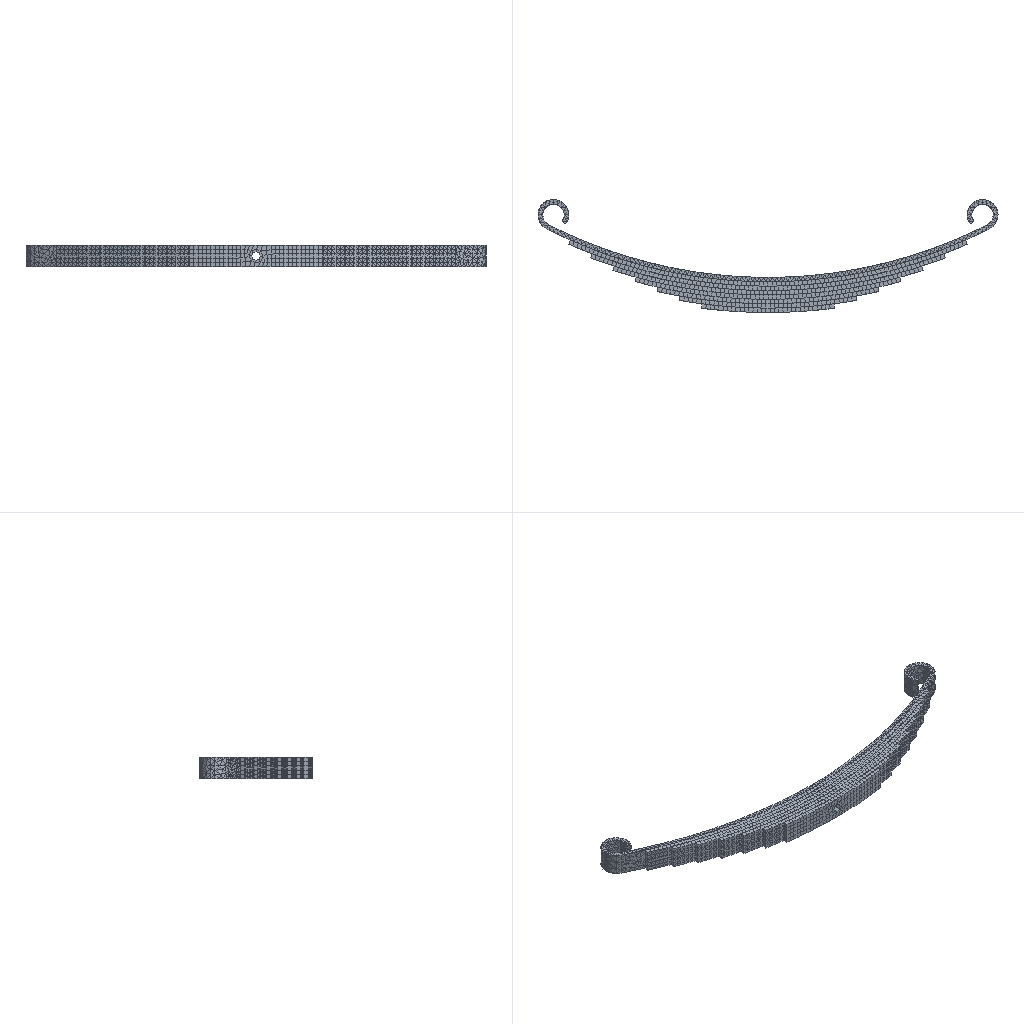Simulation study | ansys workbench
Set-up summary:
category,name,step,type,value,unit,region
solver,ansys_workbench
units,mm-N-s-tonne (MPa),,stated,"/units,MPA"
analysis,LS1,,static
load_step,LS1,LS1,static,nsubst=1; time=1
mesh,nodes,,,25414
mesh,elements,,,15995
element_type,TARGE170,,,5078
element_type,CONTA174,,,5078
element_type,SOLID187,,,3507
element_type,SOLID186,,,2176
element_type,SURF154,,,156
material,Structural Steel,,E,200000,tonne s^-2 mm^-1
material,Structural Steel,,nu,0.3
material,Structural Steel,,density,7.85e-09,tonne mm^-3
material,Structural Steel,,conductivity,60.5,tonne mm s^-3 C^-1
material,Structural Steel,,specific_heat,4.34e+08,mm^2 s^-2 C^-1
material,Structural Steel,,cte,1.2e-05,C^-1
material,Structural Steel,,permeability,10000
material,Structural Steel,,resistivity,0.00017,ohm mm
load,Define Force Using Surface Effect Elements,LS1,surface-effect pres face 2,3.366,,SURF154 #23
bc,Fixed Supports,model,fixed,[dofs=ALL],,_FIXEDSU
bc,Frictionless Supports X,model,fixed,[dofs=UX],,_FRICSUX
bc,Frictionless Supports Y,model,fixed,[dofs=UY],,_FRICSUY
bc,Frictionless Supports Z,model,fixed,[dofs=UZ],,_FRICSUZ
contact,No Separation - 8 To 7,,no separation (always),element=CONTA174
contact,No Separation - 7 To 6,,no separation (always),element=CONTA174
contact,No Separation - 6 To 5,,no separation (always),element=CONTA174
contact,No Separation - 5 To 4,,no separation (always),element=CONTA174
contact,No Separation - 4 To 3,,no separation (always),element=CONTA174
contact,No Separation - 3 To 2,,no separation (always),element=CONTA174
contact,No Separation - 2 To 1,,no separation (always),element=CONTA174
named_set,_FIXEDSU,,node,466
named_set,_FRICSUX,,node,328
named_set,_FRICSUY,,node,96
named_set,_FRICSUZ,,node,232
Ansys APDL input file, long lists of numbers shortened:
/batch
/config,noeldb,1     ! force off writing results to database
*get,_wallstrt,active,,time,wall
! ANSYS input file written by Workbench version 19.0 RELEASE
! File used for geometry attach:
/title,unsaved_project--Static Structural (A5)
*DIM,_wb_ProjectScratch_dir,string,248
_wb_ProjectScratch_dir(1) = ''
*DIM,_wb_SolverFiles_dir,string,248
_wb_SolverFiles_dir(1) = ''
*DIM,_wb_userfiles_dir,string,248
_wb_userfiles_dir(1) = ''
/com,--- Data in consistent NMM units. See Solving Units in the help system for more information.
/units,MPA
/nopr
/wb,file,start              !  signify a WB generated input file
/prep7
! Turn off shape checking because checks already performed inside WB mesher.
! See help system for more information.
SHPP,OFF,,NOWARN
/nolist
etcon,set             ! allow ANSYS to choose best KEYOP's for 180x elements
/com,*********** Nodes for the whole assembly ***********
nblock,3,,27955
(1i9,3e20.9e3)
        1    2.672589323E+001   -5.969305683E+001   -5.813771560E+000
! (25413 more lines like these left out)
-1
/wb,elem,start            !  set before creation of elements
/com,*********** Elements for Body 1 "8" ***********
et,1,186
keyo,1,2,1          ! set full integration on SOLID186
eblock,19,solid,,156
(19i9)
        1        1        1        1        0        0        0        0       20        0      207     1697     1698     1718     1761     1920     1919     1899     1856
! (311 more lines like these left out)
-1
/com,*********** Elements for Body 2 "7" ***********
et,2,186
keyo,2,2,1          ! set full integration on SOLID186
eblock,19,solid,,206
(19i9)
        2        2        2        2        0        0        0        0       20        0        1        5        6       31       89      308      307      282      224
! (411 more lines like these left out)
-1
/com,*********** Elements for Body 3 "6" ***********
et,3,186
keyo,3,2,1          ! set full integration on SOLID186
eblock,19,solid,,256
(19i9)
        3        3        3        3        0        0        0        0       20        0     1033     8429     8430     8460     8533     8812     8811     8781     8708
! (511 more lines like these left out)
-1
/com,*********** Elements for Body 4 "5" ***********
et,4,186
keyo,4,2,1          ! set full integration on SOLID186
eblock,19,solid,,312
(19i9)
        4        4        4        4        0        0        0        0       20        0      363     2992     3028     3170     3748     3457     3421     3279     3465
! (623 more lines like these left out)
-1
/com,*********** Elements for Body 5 "4" ***********
et,5,186
keyo,5,2,1          ! set full integration on SOLID186
eblock,19,solid,,358
(19i9)
        5        5        5        5        0        0        0        0       20        0      675     5520     5794     5521     5665     6069     5795     6068     5924
! (715 more lines like these left out)
-1
/com,*********** Elements for Body 6 "3" ***********
et,6,186
keyo,6,2,1          ! set full integration on SOLID186
eblock,19,solid,,416
(19i9)
        6        6        6        6        0        0        0        0       20        0     4796    18236    18405    18365    18366    18877    18708    18748    18747
! (831 more lines like these left out)
-1
/com,*********** Elements for Body 7 "2" ***********
et,7,186
keyo,7,2,1          ! set full integration on SOLID186
eblock,19,solid,,472
(19i9)
        7        7        7        7        0        0        0        0       20        0     5212    21601    21605    21847    21750    22336    22332    22090    22187
! (943 more lines like these left out)
-1
/com,*********** Elements for Body 8 "1" ***********
et,8,187
eblock,19,solid,,3507
(19i9)
        8        8        8        8        0        0        0        0       10        0     1289    11163    11667    11316    11265    15185    16145    15182    15181
! (7013 more lines like these left out)
-1
/wb,elem,end               !  done creating elements
/com,*********** Send User Defined Coordinate System(s) ***********
csys,0
toffst,273.15,  ! Temperature offset from absolute zero
/com,*********** Set Reference Temperature ***********
tref,22.
/wb,mat,start              !  starting to send materials
/com,*********** Send Materials ***********
Temperature = 'TEMP' ! Temperature
MP,DENS,1,7.85e-09,	! tonne mm^-3
MP,ALPX,1,1.2e-05,	! C^-1
MP,C,1,434000000,	! mm^2 s^-2 C^-1
MP,KXX,1,60.5,	! tonne mm s^-3 C^-1
MP,RSVX,1,0.00017,	! ohm mm
MP,EX,1,200000,	! tonne s^-2 mm^-1
MP,NUXY,1,0.3,
MP,MURX,1,10000,
Temperature = 'TEMP' ! Temperature
MP,DENS,2,7.85e-09,	! tonne mm^-3
MP,ALPX,2,1.2e-05,	! C^-1
MP,C,2,434000000,	! mm^2 s^-2 C^-1
MP,KXX,2,60.5,	! tonne mm s^-3 C^-1
MP,RSVX,2,0.00017,	! ohm mm
MP,EX,2,200000,	! tonne s^-2 mm^-1
MP,NUXY,2,0.3,
MP,MURX,2,10000,
Temperature = 'TEMP' ! Temperature
MP,DENS,3,7.85e-09,	! tonne mm^-3
MP,ALPX,3,1.2e-05,	! C^-1
MP,C,3,434000000,	! mm^2 s^-2 C^-1
MP,KXX,3,60.5,	! tonne mm s^-3 C^-1
MP,RSVX,3,0.00017,	! ohm mm
MP,EX,3,200000,	! tonne s^-2 mm^-1
MP,NUXY,3,0.3,
MP,MURX,3,10000,
Temperature = 'TEMP' ! Temperature
MP,DENS,4,7.85e-09,	! tonne mm^-3
MP,ALPX,4,1.2e-05,	! C^-1
MP,C,4,434000000,	! mm^2 s^-2 C^-1
MP,KXX,4,60.5,	! tonne mm s^-3 C^-1
MP,RSVX,4,0.00017,	! ohm mm
MP,EX,4,200000,	! tonne s^-2 mm^-1
MP,NUXY,4,0.3,
MP,MURX,4,10000,
Temperature = 'TEMP' ! Temperature
MP,DENS,5,7.85e-09,	! tonne mm^-3
MP,ALPX,5,1.2e-05,	! C^-1
MP,C,5,434000000,	! mm^2 s^-2 C^-1
MP,KXX,5,60.5,	! tonne mm s^-3 C^-1
MP,RSVX,5,0.00017,	! ohm mm
MP,EX,5,200000,	! tonne s^-2 mm^-1
MP,NUXY,5,0.3,
MP,MURX,5,10000,
Temperature = 'TEMP' ! Temperature
MP,DENS,6,7.85e-09,	! tonne mm^-3
MP,ALPX,6,1.2e-05,	! C^-1
MP,C,6,434000000,	! mm^2 s^-2 C^-1
MP,KXX,6,60.5,	! tonne mm s^-3 C^-1
MP,RSVX,6,0.00017,	! ohm mm
MP,EX,6,200000,	! tonne s^-2 mm^-1
MP,NUXY,6,0.3,
MP,MURX,6,10000,
Temperature = 'TEMP' ! Temperature
MP,DENS,7,7.85e-09,	! tonne mm^-3
MP,ALPX,7,1.2e-05,	! C^-1
MP,C,7,434000000,	! mm^2 s^-2 C^-1
MP,KXX,7,60.5,	! tonne mm s^-3 C^-1
MP,RSVX,7,0.00017,	! ohm mm
MP,EX,7,200000,	! tonne s^-2 mm^-1
MP,NUXY,7,0.3,
MP,MURX,7,10000,
Temperature = 'TEMP' ! Temperature
MP,DENS,8,7.85e-09,	! tonne mm^-3
MP,ALPX,8,1.2e-05,	! C^-1
MP,C,8,434000000,	! mm^2 s^-2 C^-1
MP,KXX,8,60.5,	! tonne mm s^-3 C^-1
MP,RSVX,8,0.00017,	! ohm mm
MP,EX,8,200000,	! tonne s^-2 mm^-1
MP,NUXY,8,0.3,
MP,MURX,8,10000,
/wb,mat,end                !  done sending materials
!************************* Model Summary ********************
!8,	Structural Steel,	matid,	1
!7,	Structural Steel,	matid,	2
!6,	Structural Steel,	matid,	3
!5,	Structural Steel,	matid,	4
!4,	Structural Steel,	matid,	5
!3,	Structural Steel,	matid,	6
!2,	Structural Steel,	matid,	7
!1,	Structural Steel,	matid,	8
!************************* End Model Summary ********************
! get the diagonal of the bounding box. Needed later for other things
*get,_xmin,node,,mnloc,x
*get,_ymin,node,,mnloc,y
*get,_zmin,node,,mnloc,z
*get,_xmax,node,,mxloc,x
*get,_ymax,node,,mxloc,y
*get,_zmax,node,,mxloc,z
_ASMDIAG=(_xmax-_xmin)*(_xmax-_xmin)+(_ymax-_ymin)*(_ymax-_ymin)+(_zmax-_zmin)*(_zmax-_zmin)
_ASMDIAG=SQRT(_ASMDIAG)
/wb,contact,start          !  starting to send contact
/com,*********** Create Contact "No Separation - 8 To 7" ***********
/com,            Real Constant Set For Above Contact Is 10 & 9
*set,tid,10
*set,cid,9
r,tid
r,cid
et,tid,170
et,cid,174
eblock,10,,,156
(15i9)
     5684       10       10       10        0     1698     1697     1761     1718     2105     2106     2193     2111
! (155 more lines like these left out)
-1
eblock,10,,,156
(15i9)
     5840        9        9        9        0     1698     1697     1761     1718     2105     2106     2193     2111
! (155 more lines like these left out)
-1
eblock,10,,,206
(15i9)
     5996        9       10        9        0      224      308      307      282     1204     1380     1325     1203
! (205 more lines like these left out)
-1
eblock,10,,,206
(15i9)
     6202       10        9       10        0      224      308      307      282     1204     1380     1325     1203
! (205 more lines like these left out)
-1
keyo,cid,8,2               ! auto create asymmetric contact (from Program Controlled setting)
keyo,cid,10,0              ! adjust contact stiffness each NR iteration (from Program Controlled setting)
keyo,cid,12,4              ! no separation always
keyo,cid,2,0               ! augmented Lagrange (from Program Controlled setting)
keyo,cid,4,0               ! on Gauss point (from Program Controlled setting)
keyo,cid,9,1               ! ignore initial gaps/penetration
keyo,cid,7,0               ! No Prediction
rmod,tid,3,10.         ! FKN
rmod,tid,5,0.          ! ICONT
rmod,tid,6,0.        ! PINB
rmod,tid,10,0.        ! CNOF
rmod,tid,12,0.        ! FKT
rmod,tid,36,96         ! WB DSID
rmod,cid,3,10.     ! FKN
rmod,cid,5,0.          ! ICONT
rmod,cid,6,0.        ! PINB
rmod,cid,10,0.        ! CNOF
rmod,cid,12,0.        ! FKT
rmod,cid,36,96         ! WB DSID
/com,*********** Create Contact "No Separation - 7 To 6" ***********
/com,            Real Constant Set For Above Contact Is 12 & 11
*set,tid,12
*set,cid,11
r,tid
r,cid
et,tid,170
et,cid,174
eblock,10,,,206
(15i9)
     6408       12       12       12        0        6        5       89       31      533      534      641      539
! (205 more lines like these left out)
-1
eblock,10,,,206
(15i9)
     6614       11       11       11        0        6        5       89       31      533      534      641      539
! (205 more lines like these left out)
-1
eblock,10,,,256
(15i9)
     6820       11       12       11        0     8708     8812     8811     8781     9928    10144    10079     9927
! (255 more lines like these left out)
-1
eblock,10,,,256
(15i9)
     7076       12       11       12        0     8708     8812     8811     8781     9928    10144    10079     9927
! (255 more lines like these left out)
-1
keyo,cid,8,2               ! auto create asymmetric contact (from Program Controlled setting)
keyo,cid,10,0              ! adjust contact stiffness each NR iteration (from Program Controlled setting)
keyo,cid,12,4              ! no separation always
keyo,cid,2,0               ! augmented Lagrange (from Program Controlled setting)
keyo,cid,4,0               ! on Gauss point (from Program Controlled setting)
keyo,cid,9,1               ! ignore initial gaps/penetration
keyo,cid,7,0               ! No Prediction
rmod,tid,3,10.  ! FKN
rmod,tid,5,0.          ! ICONT
rmod,tid,6,0.        ! PINB
rmod,tid,10,0.        ! CNOF
rmod,tid,12,0.        ! FKT
rmod,tid,36,99         ! WB DSID
rmod,cid,3,10.     ! FKN
rmod,cid,5,0.          ! ICONT
rmod,cid,6,0.        ! PINB
rmod,cid,10,0.        ! CNOF
rmod,cid,12,0.        ! FKT
rmod,cid,36,99         ! WB DSID
/com,*********** Create Contact "No Separation - 6 To 5" ***********
/com,            Real Constant Set For Above Contact Is 14 & 13
*set,tid,14
*set,cid,13
r,tid
r,cid
et,tid,170
et,cid,174
eblock,10,,,256
(15i9)
     7332       14       14       14        0     8430     8429     8533     8460     9077     9078     9205     9083
! (255 more lines like these left out)
-1
eblock,10,,,256
(15i9)
     7588       13       13       13        0     8430     8429     8533     8460     9077     9078     9205     9083
! (255 more lines like these left out)
-1
eblock,10,,,312
(15i9)
     7844       13       14       13        0     3464     3458     3277     3277     5082     4675     3277     4676
! (311 more lines like these left out)
-1
eblock,10,,,312
(15i9)
     8156       14       13       14        0     3464     3458     3277     3277     5082     4675     3277     4676
! (311 more lines like these left out)
-1
keyo,cid,8,2               ! auto create asymmetric contact (from Program Controlled setting)
keyo,cid,10,0              ! adjust contact stiffness each NR iteration (from Program Controlled setting)
keyo,cid,12,4              ! no separation always
keyo,cid,2,0               ! augmented Lagrange (from Program Controlled setting)
keyo,cid,4,0               ! on Gauss point (from Program Controlled setting)
keyo,cid,9,1               ! ignore initial gaps/penetration
keyo,cid,7,0               ! No Prediction
rmod,tid,3,10.    ! FKN
rmod,tid,5,0.          ! ICONT
rmod,tid,6,0.        ! PINB
rmod,tid,10,0.        ! CNOF
rmod,tid,12,0.        ! FKT
rmod,tid,36,102        ! WB DSID
rmod,cid,3,10.     ! FKN
rmod,cid,5,0.          ! ICONT
rmod,cid,6,0.        ! PINB
rmod,cid,10,0.        ! CNOF
rmod,cid,12,0.        ! FKT
rmod,cid,36,102        ! WB DSID
/com,*********** Create Contact "No Separation - 5 To 4" ***********
/com,            Real Constant Set For Above Contact Is 16 & 15
*set,tid,16
*set,cid,15
r,tid
r,cid
et,tid,170
et,cid,174
eblock,10,,,312
(15i9)
     8468       16       16       16        0     2985     3172     2991     2991     3751     3777     2991     3749
! (311 more lines like these left out)
-1
eblock,10,,,312
(15i9)
     8780       15       15       15        0     2985     3172     2991     2991     3751     3777     2991     3749
! (311 more lines like these left out)
-1
eblock,10,,,358
(15i9)
     9092       15       16       15        0     6185     6186     6067     6067     8170     7936     6067     7935
! (357 more lines like these left out)
-1
eblock,10,,,358
(15i9)
     9450       16       15       16        0     6185     6186     6067     6067     8170     7936     6067     7935
! (357 more lines like these left out)
-1
keyo,cid,8,2               ! auto create asymmetric contact (from Program Controlled setting)
keyo,cid,10,0              ! adjust contact stiffness each NR iteration (from Program Controlled setting)
keyo,cid,12,4              ! no separation always
keyo,cid,2,0               ! augmented Lagrange (from Program Controlled setting)
keyo,cid,4,0               ! on Gauss point (from Program Controlled setting)
keyo,cid,9,1               ! ignore initial gaps/penetration
keyo,cid,7,0               ! No Prediction
rmod,tid,3,10.        ! FKN
rmod,tid,5,0.          ! ICONT
rmod,tid,6,0.        ! PINB
rmod,tid,10,0.        ! CNOF
rmod,tid,12,0.        ! FKT
rmod,tid,36,105        ! WB DSID
rmod,cid,3,10.     ! FKN
rmod,cid,5,0.          ! ICONT
rmod,cid,6,0.        ! PINB
rmod,cid,10,0.        ! CNOF
rmod,cid,12,0.        ! FKT
rmod,cid,36,105        ! WB DSID
/com,*********** Create Contact "No Separation - 4 To 3" ***********
/com,            Real Constant Set For Above Contact Is 18 & 17
*set,tid,18
*set,cid,17
r,tid
r,cid
et,tid,170
et,cid,174
eblock,10,,,358
(15i9)
     9808       18       18       18        0     6285     5522     6286     6286     6414     6415     6286     8318
! (357 more lines like these left out)
-1
eblock,10,,,358
(15i9)
    10166       17       17       17        0     6285     5522     6286     6286     6414     6415     6286     8318
! (357 more lines like these left out)
-1
eblock,10,,,416
(15i9)
    10524       17       18       17        0    18609    18612    18557    18557    20454    20313    18557    20312
! (415 more lines like these left out)
-1
eblock,10,,,416
(15i9)
    10940       18       17       18        0    18609    18612    18557    18557    20454    20313    18557    20312
! (415 more lines like these left out)
-1
keyo,cid,8,2               ! auto create asymmetric contact (from Program Controlled setting)
keyo,cid,10,0              ! adjust contact stiffness each NR iteration (from Program Controlled setting)
keyo,cid,12,4              ! no separation always
keyo,cid,2,0               ! augmented Lagrange (from Program Controlled setting)
keyo,cid,4,0               ! on Gauss point (from Program Controlled setting)
keyo,cid,9,1               ! ignore initial gaps/penetration
keyo,cid,7,0               ! No Prediction
rmod,tid,3,10.      ! FKN
rmod,tid,5,0.          ! ICONT
rmod,tid,6,0.        ! PINB
rmod,tid,10,0.        ! CNOF
rmod,tid,12,0.        ! FKT
rmod,tid,36,108        ! WB DSID
rmod,cid,3,10.     ! FKN
rmod,cid,5,0.          ! ICONT
rmod,cid,6,0.        ! PINB
rmod,cid,10,0.        ! CNOF
rmod,cid,12,0.        ! FKT
rmod,cid,36,108        ! WB DSID
/com,*********** Create Contact "No Separation - 3 To 2" ***********
/com,            Real Constant Set For Above Contact Is 20 & 19
*set,tid,20
*set,cid,19
r,tid
r,cid
et,tid,170
et,cid,174
eblock,10,,,416
(15i9)
    11356       20       20       20        0    18504    18556    18501    18501    20190    20182    18501    20181
! (415 more lines like these left out)
-1
eblock,10,,,416
(15i9)
    11772       19       19       19        0    18504    18556    18501    18501    20190    20182    18501    20181
! (415 more lines like these left out)
-1
eblock,10,,,472
(15i9)
    12188       19       20       19        0    22119    22118    21970    21970    24346    23962    21970    23963
! (471 more lines like these left out)
-1
eblock,10,,,472
(15i9)
    12660       20       19       20        0    22119    22118    21970    21970    24346    23962    21970    23963
! (471 more lines like these left out)
-1
keyo,cid,8,2               ! auto create asymmetric contact (from Program Controlled setting)
keyo,cid,10,0              ! adjust contact stiffness each NR iteration (from Program Controlled setting)
keyo,cid,12,4              ! no separation always
keyo,cid,2,0               ! augmented Lagrange (from Program Controlled setting)
keyo,cid,4,0               ! on Gauss point (from Program Controlled setting)
keyo,cid,9,1               ! ignore initial gaps/penetration
keyo,cid,7,0               ! No Prediction
rmod,tid,3,10.    ! FKN
rmod,tid,5,0.          ! ICONT
rmod,tid,6,0.        ! PINB
rmod,tid,10,0.        ! CNOF
rmod,tid,12,0.        ! FKT
rmod,tid,36,111        ! WB DSID
rmod,cid,3,10.     ! FKN
rmod,cid,5,0.          ! ICONT
rmod,cid,6,0.        ! PINB
rmod,cid,10,0.        ! CNOF
rmod,cid,12,0.        ! FKT
rmod,cid,36,111        ! WB DSID
/com,*********** Create Contact "No Separation - 2 To 1" ***********
/com,            Real Constant Set For Above Contact Is 22 & 21
*set,tid,22
*set,cid,21
r,tid
r,cid
et,tid,170
et,cid,174
eblock,10,,,472
(15i9)
    13132       22       22       22        0    21818    21967    21819    21819    23595    23598    21819    23594
! (471 more lines like these left out)
-1
eblock,10,,,472
(15i9)
    13604       21       21       21        0    21818    21967    21819    21819    23595    23598    21819    23594
! (471 more lines like these left out)
-1
eblock,10,,,882
(15i9)
    14076       21       22       21        0    10869    10868    11612    11612    13936    13940    11612    13946
! (881 more lines like these left out)
-1
eblock,10,,,882
(15i9)
    14958       22       21       22        0    10869    10868    11612    11612    13936    13940    11612    13946
! (881 more lines like these left out)
-1
keyo,cid,8,2               ! auto create asymmetric contact (from Program Controlled setting)
keyo,cid,10,0              ! adjust contact stiffness each NR iteration (from Program Controlled setting)
keyo,cid,12,4              ! no separation always
keyo,cid,2,0               ! augmented Lagrange (from Program Controlled setting)
keyo,cid,4,0               ! on Gauss point (from Program Controlled setting)
keyo,cid,9,1               ! ignore initial gaps/penetration
keyo,cid,7,0               ! No Prediction
rmod,tid,3,10.      ! FKN
rmod,tid,5,0.          ! ICONT
rmod,tid,6,0.        ! PINB
rmod,tid,10,0.        ! CNOF
rmod,tid,12,0.        ! FKT
rmod,tid,36,114        ! WB DSID
rmod,cid,3,10.     ! FKN
rmod,cid,5,0.          ! ICONT
rmod,cid,6,0.        ! PINB
rmod,cid,10,0.        ! CNOF
rmod,cid,12,0.        ! FKT
rmod,cid,36,114        ! WB DSID
nsel,all
esel,all
/wb,contact,end            !  done creating contacts
/golist
/wb,load,start             !  starting to send loads
/com,*********** Fixed Supports ***********
CMBLOCK,_FIXEDSU,NODE,      466
(8i10)
     10527     10528     10529     10530     10531     10532     10533     10534
! (58 more lines like these left out)
cmsel,s,_FIXEDSU
d,all,all
nsel,all
/com,********* Frictionless Supports X *********
CMBLOCK,_FRICSUX,NODE,      328
(8i10)
       313       314       315       316       317       410       411       412
! (40 more lines like these left out)
cmsel,s,_FRICSUX
d,all,ux,0
nsel,all
/com,********* Frictionless Supports Y *********
CMBLOCK,_FRICSUY,NODE,       96
(8i10)
       314       315       317       411       414       415       417       511
! (11 more lines like these left out)
cmsel,s,_FRICSUY
d,all,uy,0
nsel,all
/com,********* Frictionless Supports Z *********
CMBLOCK,_FRICSUZ,NODE,      232
(8i10)
       313       316       410       412       413       416       510       512
! (28 more lines like these left out)
cmsel,s,_FRICSUZ
d,all,uz,0
nsel,all
/com,*********** Node Rotations ***********
nmod,314,,,,90.,0.,-90.
nmod,315,,,,90.,-90.,-90.
nmod,317,,,,-90.,0.,90.
nmod,411,,,,-90.,90.,90.
! (92 more lines like these left out)
/com,*********** Define Force Using Surface Effect Elements ***********
local,12,0,0.,0.,0.,-0.,0.,0.
csys,0
et,23,154
eblock,10,,,156
(15i9)
    15840       23       23       23       12     1856     1920     1919     1899     2596     2732     2687     2595
! (155 more lines like these left out)
-1
esel,s,type,,23
keyop,23,2,1                ! Apply load in local coordinate system
keyop,23,7,1                ! Use original area so load is constant in large deformation
keyop,23,11,2               ! Use real and not project area
esel,all
*DIM,_loadvari70x,TABLE,2,1,1,TIME,
! Time values
_loadvari70x(1,0,1) = 0.
_loadvari70x(2,0,1) = 1.
! Load values
_loadvari70x(1,1,1) = 0.
_loadvari70x(2,1,1) = 0.
*DIM,_loadvari70y,TABLE,2,1,1,TIME,
! Time values
_loadvari70y(1,0,1) = 0.
_loadvari70y(2,0,1) = 1.
! Load values
_loadvari70y(1,1,1) = 0.
_loadvari70y(2,1,1) = 3.366
*DIM,_loadvari70z,TABLE,2,1,1,TIME,
! Time values
_loadvari70z(1,0,1) = 0.
_loadvari70z(2,0,1) = 1.
! Load values
_loadvari70z(1,1,1) = 0.
_loadvari70z(2,1,1) = 0.
/gst,on,on
fini
*get,_numnode,node,0,count
*get,_numelem,elem,0,count
*get, _MAXELEMNUM, elem, 0, NUM, MAX
*get, _MAXNODENUM, node, 0, NUM, MAX
*get, _MAXELEMTYPE, etyp, 0, NUM, MAX
*get, _MAXREALCONST, real, 0, NUM, MAX
/go
/wb,load,end               !  done creating loads
/com,--- Number of total nodes = %_numnode%
/com,--- Number of contact elements = 10312
/com,--- Number of spring elements = 0
/com,--- Number of bearing elements = 0
/com,--- Number of solid elements = 5683
/com,--- Number of condensed parts = 0
/com,--- Number of total elements = %_numelem%
*get,_wallbsol,active,,time,wall
/com,****************************************************************************
/com,*************************    SOLUTION       ********************************
/com,****************************************************************************
/solu
antype,0                   ! static analysis
nlgeom,on                  ! Turn on Large Deformation Effects
eqsl,sparse,,,,,1
cntr,print,1               ! print out contact info and also make no initial contact an error
dmpoption,emat,no             ! Don't combine emat file for DANSYS
dmpoption,esav,no             ! Don't combine esav file for DANSYS
nldiag,cont,iter           ! print out contact info each equilibrium iteration
rescontrol,define,last,last,,dele	   ! Program Controlled
/com,****************************************************
/com,******************* SOLVE FOR LS 1 OF 1 ****************
esel,s,type,,23
nsle
sfe,all,1,pres,1,%_loadvari70x%
sfe,all,2,pres,1,%_loadvari70y%
sfe,all,3,pres,1,%_loadvari70z%
nsel,all
esel,all
/nopr
/gopr
autots,on                  ! Workbench Program Controlled automatic time stepping
nsub,1,10,1                ! due to presence of general nonlinear
time,1.
outres,erase
outres,all,none
outres,nsol,all
outres,rsol,all
outres,strs,all
outres,epel,all
outres,eppl,all
stabilize,off                   ! Stabilization turned OFF by user
! *********** WB SOLVE COMMAND ***********
! check interactive state
*get,ANSINTER_,active,,int
*if,ANSINTER_,ne,0,then
/eof
*endif
solve
/com *************** Write FE CONNECTORS *********
CEWRITE,file,ce,,INTE
/com,****************************************************
/com,*************** FINISHED SOLVE FOR LS 1 *************
*get,_wallasol,active,,time,wall
/nopr
*get,_numnode,node,0,count
*get,_numelem,elem,0,count
*get, _MAXELEMNUM, elem, 0, NUM, MAX
*get, _MAXNODENUM, node, 0, NUM, MAX,,,INTERNAL
*get, _MAXELEMTYPE, etyp, 0, NUM, MAX
*get, _MAXREALCONST, real, 0, NUM, MAX
/gopr
/post1
xmlo,ENCODING,ISO-8859-1
xmlo,parm
/xml,parm,xml
fini
/gopr
*get,_walldone,active,,time,wall
_preptime=(_wallbsol-_wallstrt)*3600
_solvtime=(_wallasol-_wallbsol)*3600
_posttime=(_walldone-_wallasol)*3600
_totaltim=(_walldone-_wallstrt)*3600
/wb,file,end               ! done with WB generated input
Results summary:
result,analyses[0].index,,,1
result,analyses[0].system,,,SYS
result,analyses[0].deck,,,deck.dat
result,analyses[0].solve_status,,,completed
result,analyses[0].analysis_type,,,static
result,analyses[0].physics,,,mechanical
result,analyses[0].unit_system,,,"NMM: mm, ton, N, s, mV, mA, degC"
result,analyses[0].n_sets,,,1
result,analyses[0].load_steps[0].set,set=1,,1
result,analyses[0].load_steps[0].time_or_freq,set=1,,1
result,analyses[0].load_steps[0].max_displacement_magnitude,set=1,,7.161
result,analyses[0].load_steps[0].max_von_mises_nodal,set=1,,948.448
result,analyses[0].load_steps[0].reaction_force_sum_xyz[1],set=1,,-0.008874
result,analyses[0].load_steps[0].reaction_force_sum_xyz[2],set=1,,-49999.8
result,analyses[0].load_steps[0].reaction_force_sum_xyz[3],set=1,,-0.001038